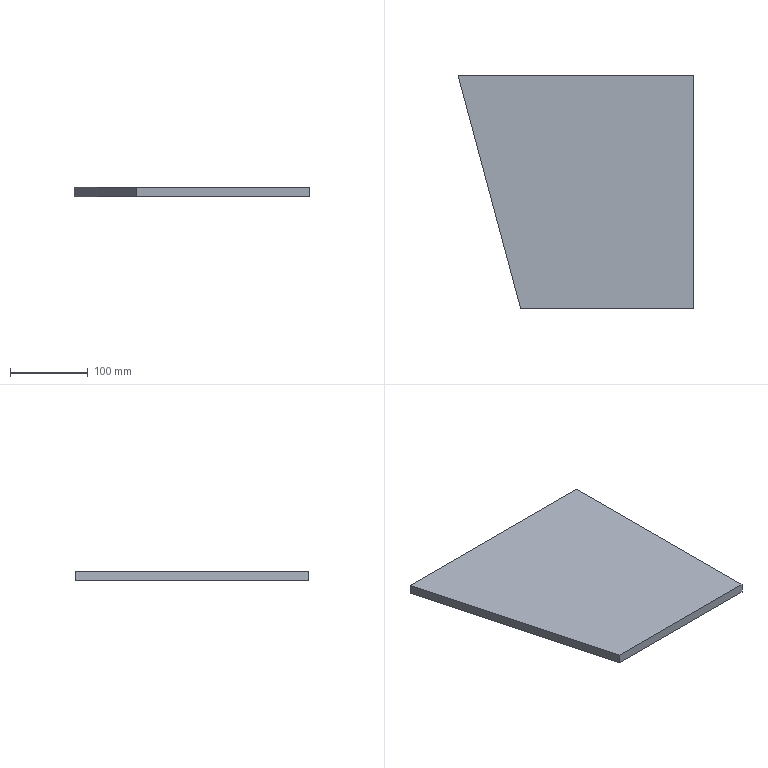Part | SolidWorks | features Extrusion 1 | 1 solid | 6 faces | box 303 x 300 x 12 mm | volume 946107 mm3 | plane 6
STEP:
#1=CARTESIAN_POINT('',(-303.,0.,-6.));
#2=VERTEX_POINT('',#1);
#3=CARTESIAN_POINT('',(-222.615,-300.,-6.));
#4=VERTEX_POINT('',#3);
#5=CARTESIAN_POINT('',(-303.,0.,-6.));
#6=DIRECTION('',(0.2588,-0.9659,0.));
#7=VECTOR('',#6,1000.);
#8=LINE('',#5,#7);
#9=EDGE_CURVE('',#2,#4,#8,.T.);
#10=ORIENTED_EDGE('',*,*,#9,.T.);
#11=CARTESIAN_POINT('',(-222.615,-300.,6.));
#12=VERTEX_POINT('',#11);
#13=CARTESIAN_POINT('',(-222.615,-300.,6.));
#14=DIRECTION('',(0.,0.,-1.));
#15=VECTOR('',#14,1000.);
#16=LINE('',#13,#15);
#17=EDGE_CURVE('',#12,#4,#16,.T.);
#18=ORIENTED_EDGE('',*,*,#17,.F.);
#19=CARTESIAN_POINT('',(-303.,0.,6.));
#20=VERTEX_POINT('',#19);
#21=CARTESIAN_POINT('',(-303.,0.,6.));
#22=DIRECTION('',(0.2588,-0.9659,0.));
#23=VECTOR('',#22,1000.);
#24=LINE('',#21,#23);
#25=EDGE_CURVE('',#20,#12,#24,.T.);
#26=ORIENTED_EDGE('',*,*,#25,.F.);
#27=CARTESIAN_POINT('',(-303.,0.,6.));
#28=DIRECTION('',(0.,0.,-1.));
#29=VECTOR('',#28,1000.);
#30=LINE('',#27,#29);
#31=EDGE_CURVE('',#20,#2,#30,.T.);
#32=ORIENTED_EDGE('',*,*,#31,.T.);
#33=EDGE_LOOP('',(#10,#18,#26,#32));
#34=FACE_OUTER_BOUND('',#33,.T.);
#35=CARTESIAN_POINT('',(-303.,0.,6.));
#36=DIRECTION('',(0.9659,0.2588,0.));
#37=DIRECTION('',(-0.2588,0.9659,0.));
#38=AXIS2_PLACEMENT_3D('',#35,#36,#37);
#39=PLANE('',#38);
#40=ADVANCED_FACE('',(#34),#39,.F.);
#41=CARTESIAN_POINT('',(0.,-300.,-6.));
#42=VERTEX_POINT('',#41);
#43=CARTESIAN_POINT('',(0.,-300.,-6.));
#44=DIRECTION('',(1.,0.,0.));
#45=VECTOR('',#44,1000.);
#46=LINE('',#43,#45);
#47=EDGE_CURVE('',#4,#42,#46,.T.);
#48=ORIENTED_EDGE('',*,*,#47,.T.);
#49=CARTESIAN_POINT('',(0.,-300.,6.));
#50=VERTEX_POINT('',#49);
#51=CARTESIAN_POINT('',(0.,-300.,6.));
#52=DIRECTION('',(0.,0.,-1.));
#53=VECTOR('',#52,1000.);
#54=LINE('',#51,#53);
#55=EDGE_CURVE('',#50,#42,#54,.T.);
#56=ORIENTED_EDGE('',*,*,#55,.F.);
#57=CARTESIAN_POINT('',(0.,-300.,6.));
#58=DIRECTION('',(1.,0.,0.));
#59=VECTOR('',#58,1000.);
#60=LINE('',#57,#59);
#61=EDGE_CURVE('',#12,#50,#60,.T.);
#62=ORIENTED_EDGE('',*,*,#61,.F.);
#63=ORIENTED_EDGE('',*,*,#17,.T.);
#64=EDGE_LOOP('',(#48,#56,#62,#63));
#65=FACE_OUTER_BOUND('',#64,.T.);
#66=CARTESIAN_POINT('',(0.,-300.,6.));
#67=DIRECTION('',(0.,1.,0.));
#68=DIRECTION('',(0.,0.,1.));
#69=AXIS2_PLACEMENT_3D('',#66,#67,#68);
#70=PLANE('',#69);
#71=ADVANCED_FACE('',(#65),#70,.F.);
#72=CARTESIAN_POINT('',(0.,0.,-6.));
#73=VERTEX_POINT('',#72);
#74=CARTESIAN_POINT('',(0.,0.,-6.));
#75=DIRECTION('',(0.,1.,0.));
#76=VECTOR('',#75,1000.);
#77=LINE('',#74,#76);
#78=EDGE_CURVE('',#42,#73,#77,.T.);
#79=ORIENTED_EDGE('',*,*,#78,.T.);
#80=CARTESIAN_POINT('',(0.,0.,6.));
#81=VERTEX_POINT('',#80);
#82=CARTESIAN_POINT('',(0.,0.,6.));
#83=DIRECTION('',(0.,0.,-1.));
#84=VECTOR('',#83,1000.);
#85=LINE('',#82,#84);
#86=EDGE_CURVE('',#81,#73,#85,.T.);
#87=ORIENTED_EDGE('',*,*,#86,.F.);
#88=CARTESIAN_POINT('',(0.,0.,6.));
#89=DIRECTION('',(0.,1.,0.));
#90=VECTOR('',#89,1000.);
#91=LINE('',#88,#90);
#92=EDGE_CURVE('',#50,#81,#91,.T.);
#93=ORIENTED_EDGE('',*,*,#92,.F.);
#94=ORIENTED_EDGE('',*,*,#55,.T.);
#95=EDGE_LOOP('',(#79,#87,#93,#94));
#96=FACE_OUTER_BOUND('',#95,.T.);
#97=CARTESIAN_POINT('',(0.,0.,6.));
#98=DIRECTION('',(-1.,0.,0.));
#99=DIRECTION('',(0.,-1.,0.));
#100=AXIS2_PLACEMENT_3D('',#97,#98,#99);
#101=PLANE('',#100);
#102=ADVANCED_FACE('',(#96),#101,.F.);
#103=CARTESIAN_POINT('',(-303.,0.,-6.));
#104=DIRECTION('',(-1.,0.,0.));
#105=VECTOR('',#104,1000.);
#106=LINE('',#103,#105);
#107=EDGE_CURVE('',#73,#2,#106,.T.);
#108=ORIENTED_EDGE('',*,*,#107,.T.);
#109=ORIENTED_EDGE('',*,*,#31,.F.);
#110=CARTESIAN_POINT('',(-303.,0.,6.));
#111=DIRECTION('',(-1.,0.,0.));
#112=VECTOR('',#111,1000.);
#113=LINE('',#110,#112);
#114=EDGE_CURVE('',#81,#20,#113,.T.);
#115=ORIENTED_EDGE('',*,*,#114,.F.);
#116=ORIENTED_EDGE('',*,*,#86,.T.);
#117=EDGE_LOOP('',(#108,#109,#115,#116));
#118=FACE_OUTER_BOUND('',#117,.T.);
#119=CARTESIAN_POINT('',(-303.,0.,6.));
#120=DIRECTION('',(0.,-1.,0.));
#121=DIRECTION('',(0.,0.,-1.));
#122=AXIS2_PLACEMENT_3D('',#119,#120,#121);
#123=PLANE('',#122);
#124=ADVANCED_FACE('',(#118),#123,.F.);
#125=ORIENTED_EDGE('',*,*,#25,.T.);
#126=ORIENTED_EDGE('',*,*,#61,.T.);
#127=ORIENTED_EDGE('',*,*,#92,.T.);
#128=ORIENTED_EDGE('',*,*,#114,.T.);
#129=EDGE_LOOP('',(#125,#126,#127,#128));
#130=FACE_OUTER_BOUND('',#129,.T.);
#131=CARTESIAN_POINT('',(-222.615,-300.,6.));
#132=DIRECTION('',(0.,0.,-1.));
#133=DIRECTION('',(-1.,0.,0.));
#134=AXIS2_PLACEMENT_3D('',#131,#132,#133);
#135=PLANE('',#134);
#136=ADVANCED_FACE('',(#130),#135,.F.);
#137=ORIENTED_EDGE('',*,*,#9,.F.);
#138=ORIENTED_EDGE('',*,*,#107,.F.);
#139=ORIENTED_EDGE('',*,*,#78,.F.);
#140=ORIENTED_EDGE('',*,*,#47,.F.);
#141=EDGE_LOOP('',(#137,#138,#139,#140));
#142=FACE_OUTER_BOUND('',#141,.T.);
#143=CARTESIAN_POINT('',(-222.615,-300.,-6.));
#144=DIRECTION('',(0.,0.,-1.));
#145=DIRECTION('',(-1.,0.,0.));
#146=AXIS2_PLACEMENT_3D('',#143,#144,#145);
#147=PLANE('',#146);
#148=ADVANCED_FACE('',(#142),#147,.T.);
#149=CLOSED_SHELL('',(#40,#71,#102,#124,#136,#148));
#150=MANIFOLD_SOLID_BREP('',#149);
#151=CARTESIAN_POINT('',(0.,0.,0.));
#152=DIRECTION('',(0.,0.,1.));
#153=DIRECTION('',(1.,0.,0.));
#154=AXIS2_PLACEMENT_3D('',#151,#152,#153);
#155=(LENGTH_UNIT()NAMED_UNIT(*)SI_UNIT(.MILLI.,.METRE.));
#156=UNCERTAINTY_MEASURE_WITH_UNIT(LENGTH_MEASURE(0.00001),#155,'','');
#157=(NAMED_UNIT(*)PLANE_ANGLE_UNIT()SI_UNIT($,.RADIAN.));
#158=(NAMED_UNIT(*)SI_UNIT($,.STERADIAN.)SOLID_ANGLE_UNIT());
#159=(GEOMETRIC_REPRESENTATION_CONTEXT(3)GLOBAL_UNCERTAINTY_ASSIGNED_CONTEXT((#156))GLOBAL_UNIT_ASSIGNED_CONTEXT((#155,#157,#158))REPRESENTATION_CONTEXT('',''));
#160=ADVANCED_BREP_SHAPE_REPRESENTATION('',(#150,#154),#159);